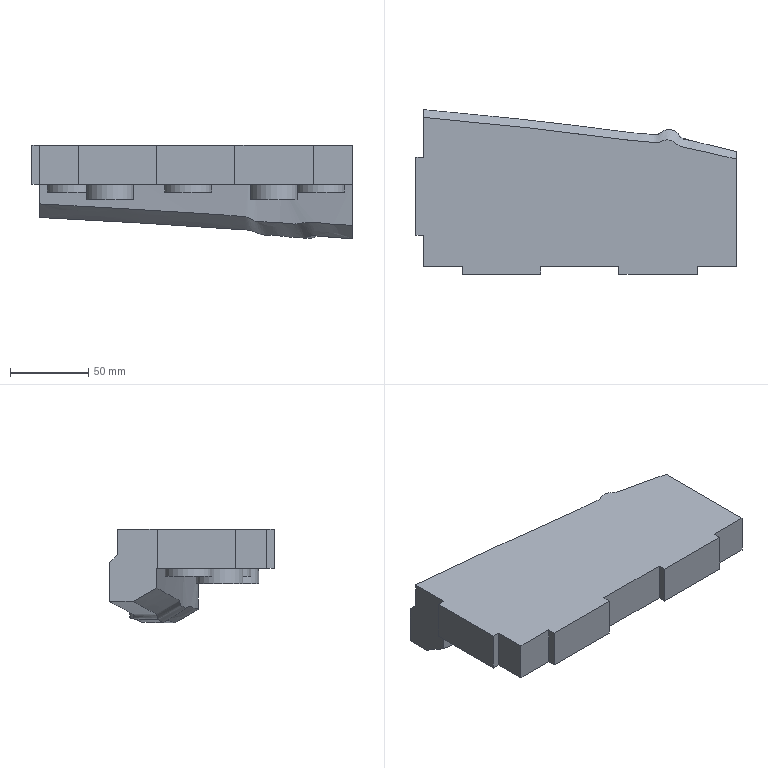Part | NX | features solid 2 | 1 solid | 35 faces | box 205 x 105.393 x 59.778 mm | volume 608862 mm3 | plane 22 | spline 8 | cylinder 5 | commonest cylinder face diameters 30 x5